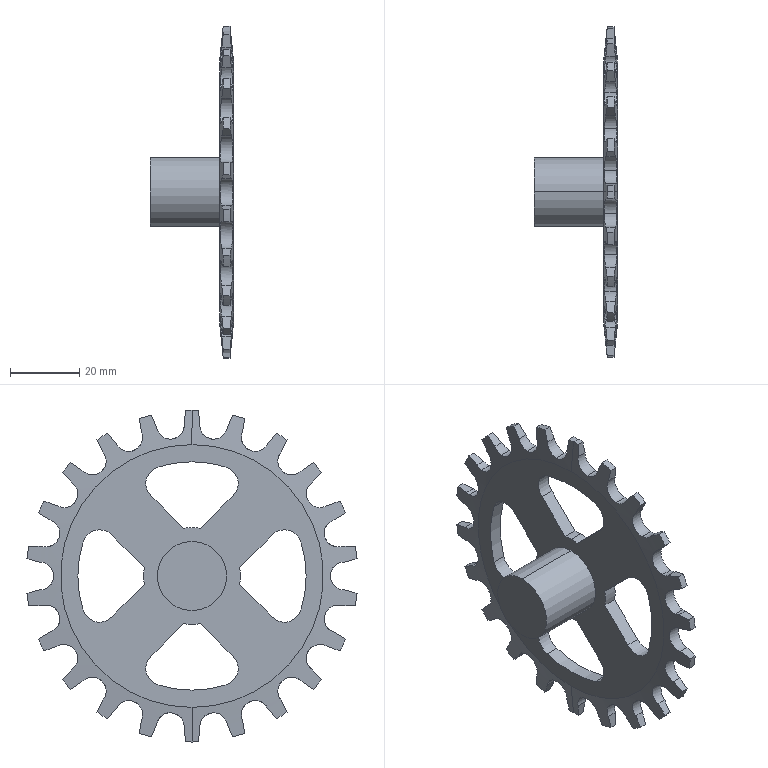Part | STEP file | Front gears inner | 1 solid | 136 faces | box 24 x 95.478 x 96 mm | volume 23028 mm3 | cylinder 77 | plane 55 | cone 4 | commonest cylinder face diameters 8 x32 96 x23 10 x10 28 x5 66 x5 20 x2